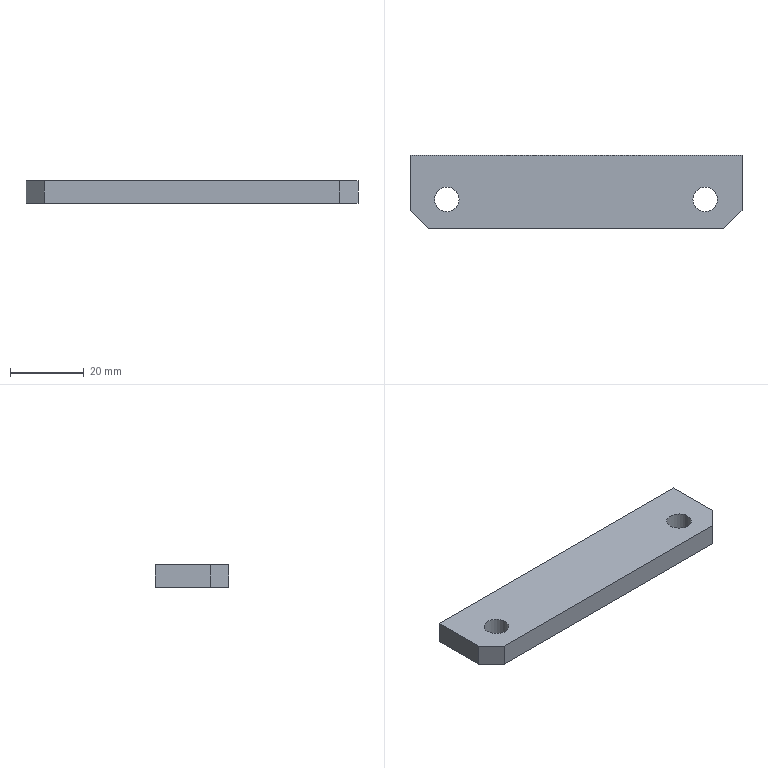Part | STEP file | weldment back plate | 1 solid | 10 faces | box 90 x 20 x 6 mm | volume 10234 mm3 | plane 8 | spline 2
STEP:
#1=CARTESIAN_POINT('',(0.,0.,0.));
#2=DIRECTION('',(0.,0.,1.));
#3=DIRECTION('',(1.,0.,0.));
#4=AXIS2_PLACEMENT_3D('',#1,#2,#3);
#5=CARTESIAN_POINT('',(90.,-15.,6.));
#6=VERTEX_POINT('',#5);
#7=CARTESIAN_POINT('',(85.,-20.,6.));
#8=VERTEX_POINT('',#7);
#9=CARTESIAN_POINT('',(90.,-15.,6.));
#10=DIRECTION('',(-0.7071,-0.7071,0.));
#11=VECTOR('',#10,1.);
#12=LINE('',#9,#11);
#13=CARTESIAN_POINT('',(87.5,-17.5,0.));
#14=DIRECTION('',(0.7071,-0.7071,0.));
#15=DIRECTION('',(0.,0.,-1.));
#16=AXIS2_PLACEMENT_3D('',#13,#14,#15);
#17=PLANE('',#16);
#18=CARTESIAN_POINT('',(-6.,3.536));
#19=DIRECTION('',(0.,-1.));
#20=VECTOR('',#19,1.);
#21=LINE('',#18,#20);
#22=(GEOMETRIC_REPRESENTATION_CONTEXT(2)PARAMETRIC_REPRESENTATION_CONTEXT()REPRESENTATION_CONTEXT('',''));
#23=DEFINITIONAL_REPRESENTATION('',(#21),#22);
#24=PCURVE('',#17,#23);
#25=CARTESIAN_POINT('',(45.,-10.,6.));
#26=DIRECTION('',(0.,0.,1.));
#27=DIRECTION('',(1.,0.,0.));
#28=AXIS2_PLACEMENT_3D('',#25,#26,#27);
#29=PLANE('',#28);
#30=CARTESIAN_POINT('',(45.,-5.));
#31=DIRECTION('',(-0.7071,-0.7071));
#32=VECTOR('',#31,1.);
#33=LINE('',#30,#32);
#34=(GEOMETRIC_REPRESENTATION_CONTEXT(2)PARAMETRIC_REPRESENTATION_CONTEXT()REPRESENTATION_CONTEXT('',''));
#35=DEFINITIONAL_REPRESENTATION('',(#33),#34);
#36=PCURVE('',#29,#35);
#37=SURFACE_CURVE('',#12,(#24,#36),.PCURVE_S1.);
#38=EDGE_CURVE('',#6,#8,#37,.T.);
#39=ORIENTED_EDGE('',*,*,#38,.T.);
#40=CARTESIAN_POINT('',(85.,-20.,0.));
#41=VERTEX_POINT('',#40);
#42=CARTESIAN_POINT('',(85.,-20.,6.));
#43=DIRECTION('',(0.,0.,-1.));
#44=VECTOR('',#43,1.);
#45=LINE('',#42,#44);
#46=CARTESIAN_POINT('',(-6.,-3.536));
#47=DIRECTION('',(1.,0.));
#48=VECTOR('',#47,1.);
#49=LINE('',#46,#48);
#50=(GEOMETRIC_REPRESENTATION_CONTEXT(2)PARAMETRIC_REPRESENTATION_CONTEXT()REPRESENTATION_CONTEXT('',''));
#51=DEFINITIONAL_REPRESENTATION('',(#49),#50);
#52=PCURVE('',#17,#51);
#53=CARTESIAN_POINT('',(90.,-20.,0.));
#54=DIRECTION('',(0.,-1.,0.));
#55=DIRECTION('',(0.,0.,-1.));
#56=AXIS2_PLACEMENT_3D('',#53,#54,#55);
#57=PLANE('',#56);
#58=CARTESIAN_POINT('',(-6.,-5.));
#59=DIRECTION('',(1.,0.));
#60=VECTOR('',#59,1.);
#61=LINE('',#58,#60);
#62=(GEOMETRIC_REPRESENTATION_CONTEXT(2)PARAMETRIC_REPRESENTATION_CONTEXT()REPRESENTATION_CONTEXT('',''));
#63=DEFINITIONAL_REPRESENTATION('',(#61),#62);
#64=PCURVE('',#57,#63);
#65=SURFACE_CURVE('',#45,(#52,#64),.PCURVE_S1.);
#66=EDGE_CURVE('',#8,#41,#65,.T.);
#67=ORIENTED_EDGE('',*,*,#66,.T.);
#68=CARTESIAN_POINT('',(90.,-15.,0.));
#69=VERTEX_POINT('',#68);
#70=CARTESIAN_POINT('',(85.,-20.,0.));
#71=DIRECTION('',(0.7071,0.7071,0.));
#72=VECTOR('',#71,1.);
#73=LINE('',#70,#72);
#74=CARTESIAN_POINT('',(0.,-3.536));
#75=DIRECTION('',(0.,1.));
#76=VECTOR('',#75,1.);
#77=LINE('',#74,#76);
#78=(GEOMETRIC_REPRESENTATION_CONTEXT(2)PARAMETRIC_REPRESENTATION_CONTEXT()REPRESENTATION_CONTEXT('',''));
#79=DEFINITIONAL_REPRESENTATION('',(#77),#78);
#80=PCURVE('',#17,#79);
#81=CARTESIAN_POINT('',(45.,-10.,0.));
#82=DIRECTION('',(0.,0.,1.));
#83=DIRECTION('',(1.,0.,0.));
#84=AXIS2_PLACEMENT_3D('',#81,#82,#83);
#85=PLANE('',#84);
#86=CARTESIAN_POINT('',(40.,-10.));
#87=DIRECTION('',(0.7071,0.7071));
#88=VECTOR('',#87,1.);
#89=LINE('',#86,#88);
#90=(GEOMETRIC_REPRESENTATION_CONTEXT(2)PARAMETRIC_REPRESENTATION_CONTEXT()REPRESENTATION_CONTEXT('',''));
#91=DEFINITIONAL_REPRESENTATION('',(#89),#90);
#92=PCURVE('',#85,#91);
#93=SURFACE_CURVE('',#73,(#80,#92),.PCURVE_S1.);
#94=EDGE_CURVE('',#41,#69,#93,.T.);
#95=ORIENTED_EDGE('',*,*,#94,.T.);
#96=CARTESIAN_POINT('',(90.,-15.,0.));
#97=DIRECTION('',(0.,0.,1.));
#98=VECTOR('',#97,1.);
#99=LINE('',#96,#98);
#100=CARTESIAN_POINT('',(0.,3.536));
#101=DIRECTION('',(-1.,0.));
#102=VECTOR('',#101,1.);
#103=LINE('',#100,#102);
#104=(GEOMETRIC_REPRESENTATION_CONTEXT(2)PARAMETRIC_REPRESENTATION_CONTEXT()REPRESENTATION_CONTEXT('',''));
#105=DEFINITIONAL_REPRESENTATION('',(#103),#104);
#106=PCURVE('',#17,#105);
#107=CARTESIAN_POINT('',(90.,0.,0.));
#108=DIRECTION('',(1.,0.,0.));
#109=DIRECTION('',(0.,0.,-1.));
#110=AXIS2_PLACEMENT_3D('',#107,#108,#109);
#111=PLANE('',#110);
#112=CARTESIAN_POINT('',(0.,-15.));
#113=DIRECTION('',(-1.,0.));
#114=VECTOR('',#113,1.);
#115=LINE('',#112,#114);
#116=(GEOMETRIC_REPRESENTATION_CONTEXT(2)PARAMETRIC_REPRESENTATION_CONTEXT()REPRESENTATION_CONTEXT('',''));
#117=DEFINITIONAL_REPRESENTATION('',(#115),#116);
#118=PCURVE('',#111,#117);
#119=SURFACE_CURVE('',#99,(#106,#118),.PCURVE_S1.);
#120=EDGE_CURVE('',#69,#6,#119,.T.);
#121=ORIENTED_EDGE('',*,*,#120,.T.);
#122=EDGE_LOOP('',(#39,#67,#95,#121));
#123=FACE_BOUND('',#122,.T.);
#124=ADVANCED_FACE('',(#123),#17,.T.);
#125=ORIENTED_EDGE('',*,*,#120,.F.);
#126=CARTESIAN_POINT('',(90.,0.,0.));
#127=VERTEX_POINT('',#126);
#128=CARTESIAN_POINT('',(90.,0.,0.));
#129=DIRECTION('',(0.,-1.,0.));
#130=VECTOR('',#129,1.);
#131=LINE('',#128,#130);
#132=CARTESIAN_POINT('',(0.,0.));
#133=DIRECTION('',(0.,-1.));
#134=VECTOR('',#133,1.);
#135=LINE('',#132,#134);
#136=(GEOMETRIC_REPRESENTATION_CONTEXT(2)PARAMETRIC_REPRESENTATION_CONTEXT()REPRESENTATION_CONTEXT('',''));
#137=DEFINITIONAL_REPRESENTATION('',(#135),#136);
#138=PCURVE('',#111,#137);
#139=CARTESIAN_POINT('',(45.,10.));
#140=DIRECTION('',(0.,-1.));
#141=VECTOR('',#140,1.);
#142=LINE('',#139,#141);
#143=(GEOMETRIC_REPRESENTATION_CONTEXT(2)PARAMETRIC_REPRESENTATION_CONTEXT()REPRESENTATION_CONTEXT('',''));
#144=DEFINITIONAL_REPRESENTATION('',(#142),#143);
#145=PCURVE('',#85,#144);
#146=SURFACE_CURVE('',#131,(#138,#145),.PCURVE_S1.);
#147=EDGE_CURVE('',#127,#69,#146,.T.);
#148=ORIENTED_EDGE('',*,*,#147,.F.);
#149=CARTESIAN_POINT('',(90.,0.,6.));
#150=VERTEX_POINT('',#149);
#151=CARTESIAN_POINT('',(90.,0.,0.));
#152=DIRECTION('',(0.,0.,1.));
#153=VECTOR('',#152,1.);
#154=LINE('',#151,#153);
#155=CARTESIAN_POINT('',(0.,0.));
#156=DIRECTION('',(-1.,0.));
#157=VECTOR('',#156,1.);
#158=LINE('',#155,#157);
#159=(GEOMETRIC_REPRESENTATION_CONTEXT(2)PARAMETRIC_REPRESENTATION_CONTEXT()REPRESENTATION_CONTEXT('',''));
#160=DEFINITIONAL_REPRESENTATION('',(#158),#159);
#161=PCURVE('',#111,#160);
#162=CARTESIAN_POINT('',(0.,0.,0.));
#163=DIRECTION('',(0.,1.,0.));
#164=DIRECTION('',(0.,0.,1.));
#165=AXIS2_PLACEMENT_3D('',#162,#163,#164);
#166=PLANE('',#165);
#167=CARTESIAN_POINT('',(0.,90.));
#168=DIRECTION('',(1.,0.));
#169=VECTOR('',#168,1.);
#170=LINE('',#167,#169);
#171=(GEOMETRIC_REPRESENTATION_CONTEXT(2)PARAMETRIC_REPRESENTATION_CONTEXT()REPRESENTATION_CONTEXT('',''));
#172=DEFINITIONAL_REPRESENTATION('',(#170),#171);
#173=PCURVE('',#166,#172);
#174=SURFACE_CURVE('',#154,(#161,#173),.PCURVE_S1.);
#175=EDGE_CURVE('',#127,#150,#174,.T.);
#176=ORIENTED_EDGE('',*,*,#175,.T.);
#177=CARTESIAN_POINT('',(90.,0.,6.));
#178=DIRECTION('',(0.,-1.,0.));
#179=VECTOR('',#178,1.);
#180=LINE('',#177,#179);
#181=CARTESIAN_POINT('',(-6.,0.));
#182=DIRECTION('',(0.,-1.));
#183=VECTOR('',#182,1.);
#184=LINE('',#181,#183);
#185=(GEOMETRIC_REPRESENTATION_CONTEXT(2)PARAMETRIC_REPRESENTATION_CONTEXT()REPRESENTATION_CONTEXT('',''));
#186=DEFINITIONAL_REPRESENTATION('',(#184),#185);
#187=PCURVE('',#111,#186);
#188=CARTESIAN_POINT('',(45.,10.));
#189=DIRECTION('',(0.,-1.));
#190=VECTOR('',#189,1.);
#191=LINE('',#188,#190);
#192=(GEOMETRIC_REPRESENTATION_CONTEXT(2)PARAMETRIC_REPRESENTATION_CONTEXT()REPRESENTATION_CONTEXT('',''));
#193=DEFINITIONAL_REPRESENTATION('',(#191),#192);
#194=PCURVE('',#29,#193);
#195=SURFACE_CURVE('',#180,(#187,#194),.PCURVE_S1.);
#196=EDGE_CURVE('',#150,#6,#195,.T.);
#197=ORIENTED_EDGE('',*,*,#196,.T.);
#198=EDGE_LOOP('',(#125,#148,#176,#197));
#199=FACE_BOUND('',#198,.T.);
#200=ADVANCED_FACE('',(#199),#111,.T.);
#201=ORIENTED_EDGE('',*,*,#94,.F.);
#202=CARTESIAN_POINT('',(5.,-20.,0.));
#203=VERTEX_POINT('',#202);
#204=CARTESIAN_POINT('',(85.,-20.,0.));
#205=DIRECTION('',(-1.,0.,0.));
#206=VECTOR('',#205,1.);
#207=LINE('',#204,#206);
#208=CARTESIAN_POINT('',(40.,-10.));
#209=DIRECTION('',(-1.,0.));
#210=VECTOR('',#209,1.);
#211=LINE('',#208,#210);
#212=(GEOMETRIC_REPRESENTATION_CONTEXT(2)PARAMETRIC_REPRESENTATION_CONTEXT()REPRESENTATION_CONTEXT('',''));
#213=DEFINITIONAL_REPRESENTATION('',(#211),#212);
#214=PCURVE('',#85,#213);
#215=CARTESIAN_POINT('',(0.,-5.));
#216=DIRECTION('',(0.,-1.));
#217=VECTOR('',#216,1.);
#218=LINE('',#215,#217);
#219=(GEOMETRIC_REPRESENTATION_CONTEXT(2)PARAMETRIC_REPRESENTATION_CONTEXT()REPRESENTATION_CONTEXT('',''));
#220=DEFINITIONAL_REPRESENTATION('',(#218),#219);
#221=PCURVE('',#57,#220);
#222=SURFACE_CURVE('',#207,(#214,#221),.PCURVE_S1.);
#223=EDGE_CURVE('',#41,#203,#222,.T.);
#224=ORIENTED_EDGE('',*,*,#223,.T.);
#225=CARTESIAN_POINT('',(0.,-15.,0.));
#226=VERTEX_POINT('',#225);
#227=CARTESIAN_POINT('',(0.,-15.,0.));
#228=DIRECTION('',(0.7071,-0.7071,0.));
#229=VECTOR('',#228,1.);
#230=LINE('',#227,#229);
#231=CARTESIAN_POINT('',(-45.,-5.));
#232=DIRECTION('',(0.7071,-0.7071));
#233=VECTOR('',#232,1.);
#234=LINE('',#231,#233);
#235=(GEOMETRIC_REPRESENTATION_CONTEXT(2)PARAMETRIC_REPRESENTATION_CONTEXT()REPRESENTATION_CONTEXT('',''));
#236=DEFINITIONAL_REPRESENTATION('',(#234),#235);
#237=PCURVE('',#85,#236);
#238=CARTESIAN_POINT('',(2.5,-17.5,0.));
#239=DIRECTION('',(-0.7071,-0.7071,0.));
#240=DIRECTION('',(0.,0.,1.));
#241=AXIS2_PLACEMENT_3D('',#238,#239,#240);
#242=PLANE('',#241);
#243=CARTESIAN_POINT('',(0.,3.536));
#244=DIRECTION('',(0.,-1.));
#245=VECTOR('',#244,1.);
#246=LINE('',#243,#245);
#247=(GEOMETRIC_REPRESENTATION_CONTEXT(2)PARAMETRIC_REPRESENTATION_CONTEXT()REPRESENTATION_CONTEXT('',''));
#248=DEFINITIONAL_REPRESENTATION('',(#246),#247);
#249=PCURVE('',#242,#248);
#250=SURFACE_CURVE('',#230,(#237,#249),.PCURVE_S1.);
#251=EDGE_CURVE('',#226,#203,#250,.T.);
#252=ORIENTED_EDGE('',*,*,#251,.F.);
#253=CARTESIAN_POINT('',(0.,0.,0.));
#254=VERTEX_POINT('',#253);
#255=CARTESIAN_POINT('',(0.,-15.,0.));
#256=DIRECTION('',(0.,1.,0.));
#257=VECTOR('',#256,1.);
#258=LINE('',#255,#257);
#259=CARTESIAN_POINT('',(-45.,-5.));
#260=DIRECTION('',(0.,1.));
#261=VECTOR('',#260,1.);
#262=LINE('',#259,#261);
#263=(GEOMETRIC_REPRESENTATION_CONTEXT(2)PARAMETRIC_REPRESENTATION_CONTEXT()REPRESENTATION_CONTEXT('',''));
#264=DEFINITIONAL_REPRESENTATION('',(#262),#263);
#265=PCURVE('',#85,#264);
#266=CARTESIAN_POINT('',(0.,-20.,0.));
#267=DIRECTION('',(-1.,0.,0.));
#268=DIRECTION('',(0.,0.,1.));
#269=AXIS2_PLACEMENT_3D('',#266,#267,#268);
#270=PLANE('',#269);
#271=CARTESIAN_POINT('',(0.,5.));
#272=DIRECTION('',(0.,1.));
#273=VECTOR('',#272,1.);
#274=LINE('',#271,#273);
#275=(GEOMETRIC_REPRESENTATION_CONTEXT(2)PARAMETRIC_REPRESENTATION_CONTEXT()REPRESENTATION_CONTEXT('',''));
#276=DEFINITIONAL_REPRESENTATION('',(#274),#275);
#277=PCURVE('',#270,#276);
#278=SURFACE_CURVE('',#258,(#265,#277),.PCURVE_S1.);
#279=EDGE_CURVE('',#226,#254,#278,.T.);
#280=ORIENTED_EDGE('',*,*,#279,.T.);
#281=CARTESIAN_POINT('',(0.,0.,0.));
#282=DIRECTION('',(1.,0.,0.));
#283=VECTOR('',#282,1.);
#284=LINE('',#281,#283);
#285=CARTESIAN_POINT('',(-45.,10.));
#286=DIRECTION('',(1.,0.));
#287=VECTOR('',#286,1.);
#288=LINE('',#285,#287);
#289=(GEOMETRIC_REPRESENTATION_CONTEXT(2)PARAMETRIC_REPRESENTATION_CONTEXT()REPRESENTATION_CONTEXT('',''));
#290=DEFINITIONAL_REPRESENTATION('',(#288),#289);
#291=PCURVE('',#85,#290);
#292=CARTESIAN_POINT('',(0.,0.));
#293=DIRECTION('',(0.,1.));
#294=VECTOR('',#293,1.);
#295=LINE('',#292,#294);
#296=(GEOMETRIC_REPRESENTATION_CONTEXT(2)PARAMETRIC_REPRESENTATION_CONTEXT()REPRESENTATION_CONTEXT('',''));
#297=DEFINITIONAL_REPRESENTATION('',(#295),#296);
#298=PCURVE('',#166,#297);
#299=SURFACE_CURVE('',#284,(#291,#298),.PCURVE_S1.);
#300=EDGE_CURVE('',#254,#127,#299,.T.);
#301=ORIENTED_EDGE('',*,*,#300,.T.);
#302=ORIENTED_EDGE('',*,*,#147,.T.);
#303=EDGE_LOOP('',(#201,#224,#252,#280,#301,#302));
#304=FACE_BOUND('',#303,.T.);
#305=CARTESIAN_POINT('',(76.677,-12.,0.));
#306=VERTEX_POINT('',#305);
#307=CARTESIAN_POINT('',(80.,-12.,0.));
#308=DIRECTION('',(0.,0.,1.));
#309=DIRECTION('',(1.,0.,0.));
#310=AXIS2_PLACEMENT_3D('',#307,#308,#309);
#311=CIRCLE('',#310,3.324);
#312=CARTESIAN_POINT('',(35.,-2.));
#313=DIRECTION('',(1.,0.));
#314=AXIS2_PLACEMENT_2D('',#312,#313);
#315=CIRCLE('',#314,3.324);
#316=(GEOMETRIC_REPRESENTATION_CONTEXT(2)PARAMETRIC_REPRESENTATION_CONTEXT()REPRESENTATION_CONTEXT('',''));
#317=DEFINITIONAL_REPRESENTATION('',(#315),#316);
#318=PCURVE('',#85,#317);
#319=CARTESIAN_POINT('',(76.677,-12.,6.));
#320=CARTESIAN_POINT('',(76.677,-15.323,6.));
#321=CARTESIAN_POINT('',(80.,-15.323,6.));
#322=CARTESIAN_POINT('',(83.323,-15.323,6.));
#323=CARTESIAN_POINT('',(83.323,-12.,6.));
#324=CARTESIAN_POINT('',(83.323,-8.677,6.));
#325=CARTESIAN_POINT('',(80.,-8.677,6.));
#326=CARTESIAN_POINT('',(76.677,-8.677,6.));
#327=CARTESIAN_POINT('',(76.677,-12.,6.));
#328=CARTESIAN_POINT('',(76.677,-12.,0.));
#329=CARTESIAN_POINT('',(76.677,-15.323,0.));
#330=CARTESIAN_POINT('',(80.,-15.323,0.));
#331=CARTESIAN_POINT('',(83.323,-15.323,0.));
#332=CARTESIAN_POINT('',(83.323,-12.,0.));
#333=CARTESIAN_POINT('',(83.323,-8.677,0.));
#334=CARTESIAN_POINT('',(80.,-8.677,0.));
#335=CARTESIAN_POINT('',(76.677,-8.677,0.));
#336=CARTESIAN_POINT('',(76.677,-12.,0.));
#337=(BOUNDED_SURFACE()B_SPLINE_SURFACE(1,2,((#319,#320,#321,#322,#323,#324,#325,#326,#327),(#328,#329,#330,#331,#332,#333,#334,#335,#336)),.UNSPECIFIED.,.F.,.T.,.F.)B_SPLINE_SURFACE_WITH_KNOTS((2,2),(1,2,2,2,2,2,1),(-27.799,-25.994),(-5.221,0.,5.221,10.441,15.662,20.882,26.103),.UNSPECIFIED.)GEOMETRIC_REPRESENTATION_ITEM()RATIONAL_B_SPLINE_SURFACE(((1.,0.7071,1.,0.7071,1.,0.7071,1.,0.7071,1.),(1.,0.7071,1.,0.7071,1.,0.7071,1.,0.7071,1.)))REPRESENTATION_ITEM('')SURFACE());
#338=CARTESIAN_POINT('',(-25.994,0.));
#339=CARTESIAN_POINT('',(-25.994,0.3505));
#340=CARTESIAN_POINT('',(-25.994,1.014));
#341=CARTESIAN_POINT('',(-25.994,1.937));
#342=CARTESIAN_POINT('',(-25.994,2.834));
#343=CARTESIAN_POINT('',(-25.994,3.74));
#344=CARTESIAN_POINT('',(-25.994,4.688));
#345=CARTESIAN_POINT('',(-25.994,5.753));
#346=CARTESIAN_POINT('',(-25.994,6.701));
#347=CARTESIAN_POINT('',(-25.994,7.607));
#348=CARTESIAN_POINT('',(-25.994,8.505));
#349=CARTESIAN_POINT('',(-25.994,9.422));
#350=CARTESIAN_POINT('',(-25.994,10.441));
#351=CARTESIAN_POINT('',(-25.994,11.46));
#352=CARTESIAN_POINT('',(-25.994,12.377));
#353=CARTESIAN_POINT('',(-25.994,13.275));
#354=CARTESIAN_POINT('',(-25.994,14.181));
#355=CARTESIAN_POINT('',(-25.994,15.129));
#356=CARTESIAN_POINT('',(-25.994,16.194));
#357=CARTESIAN_POINT('',(-25.994,17.142));
#358=CARTESIAN_POINT('',(-25.994,18.049));
#359=CARTESIAN_POINT('',(-25.994,18.945));
#360=CARTESIAN_POINT('',(-25.994,19.868));
#361=CARTESIAN_POINT('',(-25.994,20.532));
#362=CARTESIAN_POINT('',(-25.994,20.882));
#363=B_SPLINE_CURVE_WITH_KNOTS('',3,(#338,#339,#340,#341,#342,#343,#344,#345,#346,#347,#348,#349,#350,#351,#352,#353,#354,#355,#356,#357,#358,#359,#360,#361,#362),.UNSPECIFIED.,.F.,.F.,(4,1,1,1,1,1,1,1,1,1,1,1,1,1,1,1,1,1,1,1,1,1,4),(3.142,3.427,3.713,3.998,4.284,4.57,4.855,5.141,5.426,5.712,5.998,6.283,6.569,6.854,7.14,7.426,7.711,7.997,8.282,8.568,8.854,9.139,9.425),.QUASI_UNIFORM_KNOTS.);
#364=(GEOMETRIC_REPRESENTATION_CONTEXT(2)PARAMETRIC_REPRESENTATION_CONTEXT()REPRESENTATION_CONTEXT('',''));
#365=DEFINITIONAL_REPRESENTATION('',(#363),#364);
#366=PCURVE('',#337,#365);
#367=SURFACE_CURVE('',#311,(#318,#366),.PCURVE_S1.);
#368=EDGE_CURVE('',#306,#306,#367,.T.);
#369=ORIENTED_EDGE('',*,*,#368,.T.);
#370=EDGE_LOOP('',(#369));
#371=FACE_BOUND('',#370,.T.);
#372=CARTESIAN_POINT('',(6.676,-12.,0.));
#373=VERTEX_POINT('',#372);
#374=CARTESIAN_POINT('',(10.,-12.,0.));
#375=DIRECTION('',(0.,0.,1.));
#376=DIRECTION('',(1.,0.,0.));
#377=AXIS2_PLACEMENT_3D('',#374,#375,#376);
#378=CIRCLE('',#377,3.324);
#379=CARTESIAN_POINT('',(-35.,-2.));
#380=DIRECTION('',(1.,0.));
#381=AXIS2_PLACEMENT_2D('',#379,#380);
#382=CIRCLE('',#381,3.324);
#383=(GEOMETRIC_REPRESENTATION_CONTEXT(2)PARAMETRIC_REPRESENTATION_CONTEXT()REPRESENTATION_CONTEXT('',''));
#384=DEFINITIONAL_REPRESENTATION('',(#382),#383);
#385=PCURVE('',#85,#384);
#386=CARTESIAN_POINT('',(6.676,-12.,6.));
#387=CARTESIAN_POINT('',(6.676,-15.323,6.));
#388=CARTESIAN_POINT('',(10.,-15.323,6.));
#389=CARTESIAN_POINT('',(13.323,-15.323,6.));
#390=CARTESIAN_POINT('',(13.323,-12.,6.));
#391=CARTESIAN_POINT('',(13.323,-8.677,6.));
#392=CARTESIAN_POINT('',(10.,-8.677,6.));
#393=CARTESIAN_POINT('',(6.676,-8.677,6.));
#394=CARTESIAN_POINT('',(6.676,-12.,6.));
#395=CARTESIAN_POINT('',(6.676,-12.,0.));
#396=CARTESIAN_POINT('',(6.676,-15.323,0.));
#397=CARTESIAN_POINT('',(10.,-15.323,0.));
#398=CARTESIAN_POINT('',(13.323,-15.323,0.));
#399=CARTESIAN_POINT('',(13.323,-12.,0.));
#400=CARTESIAN_POINT('',(13.323,-8.677,0.));
#401=CARTESIAN_POINT('',(10.,-8.677,0.));
#402=CARTESIAN_POINT('',(6.676,-8.677,0.));
#403=CARTESIAN_POINT('',(6.676,-12.,0.));
#404=(BOUNDED_SURFACE()B_SPLINE_SURFACE(1,2,((#386,#387,#388,#389,#390,#391,#392,#393,#394),(#395,#396,#397,#398,#399,#400,#401,#402,#403)),.UNSPECIFIED.,.F.,.T.,.F.)B_SPLINE_SURFACE_WITH_KNOTS((2,2),(1,2,2,2,2,2,1),(-27.799,-25.994),(-5.221,0.,5.221,10.441,15.662,20.882,26.103),.UNSPECIFIED.)GEOMETRIC_REPRESENTATION_ITEM()RATIONAL_B_SPLINE_SURFACE(((1.,0.7071,1.,0.7071,1.,0.7071,1.,0.7071,1.),(1.,0.7071,1.,0.7071,1.,0.7071,1.,0.7071,1.)))REPRESENTATION_ITEM('')SURFACE());
#405=CARTESIAN_POINT('',(-25.994,0.));
#406=CARTESIAN_POINT('',(-25.994,0.3505));
#407=CARTESIAN_POINT('',(-25.994,1.014));
#408=CARTESIAN_POINT('',(-25.994,1.937));
#409=CARTESIAN_POINT('',(-25.994,2.834));
#410=CARTESIAN_POINT('',(-25.994,3.74));
#411=CARTESIAN_POINT('',(-25.994,4.688));
#412=CARTESIAN_POINT('',(-25.994,5.753));
#413=CARTESIAN_POINT('',(-25.994,6.701));
#414=CARTESIAN_POINT('',(-25.994,7.607));
#415=CARTESIAN_POINT('',(-25.994,8.505));
#416=CARTESIAN_POINT('',(-25.994,9.422));
#417=CARTESIAN_POINT('',(-25.994,10.441));
#418=CARTESIAN_POINT('',(-25.994,11.46));
#419=CARTESIAN_POINT('',(-25.994,12.377));
#420=CARTESIAN_POINT('',(-25.994,13.275));
#421=CARTESIAN_POINT('',(-25.994,14.181));
#422=CARTESIAN_POINT('',(-25.994,15.129));
#423=CARTESIAN_POINT('',(-25.994,16.194));
#424=CARTESIAN_POINT('',(-25.994,17.142));
#425=CARTESIAN_POINT('',(-25.994,18.049));
#426=CARTESIAN_POINT('',(-25.994,18.945));
#427=CARTESIAN_POINT('',(-25.994,19.868));
#428=CARTESIAN_POINT('',(-25.994,20.532));
#429=CARTESIAN_POINT('',(-25.994,20.882));
#430=B_SPLINE_CURVE_WITH_KNOTS('',3,(#405,#406,#407,#408,#409,#410,#411,#412,#413,#414,#415,#416,#417,#418,#419,#420,#421,#422,#423,#424,#425,#426,#427,#428,#429),.UNSPECIFIED.,.F.,.F.,(4,1,1,1,1,1,1,1,1,1,1,1,1,1,1,1,1,1,1,1,1,1,4),(3.142,3.427,3.713,3.998,4.284,4.57,4.855,5.141,5.426,5.712,5.998,6.283,6.569,6.854,7.14,7.426,7.711,7.997,8.282,8.568,8.854,9.139,9.425),.QUASI_UNIFORM_KNOTS.);
#431=(GEOMETRIC_REPRESENTATION_CONTEXT(2)PARAMETRIC_REPRESENTATION_CONTEXT()REPRESENTATION_CONTEXT('',''));
#432=DEFINITIONAL_REPRESENTATION('',(#430),#431);
#433=PCURVE('',#404,#432);
#434=SURFACE_CURVE('',#378,(#385,#433),.PCURVE_S1.);
#435=EDGE_CURVE('',#373,#373,#434,.T.);
#436=ORIENTED_EDGE('',*,*,#435,.T.);
#437=EDGE_LOOP('',(#436));
#438=FACE_BOUND('',#437,.T.);
#439=ADVANCED_FACE('',(#304,#371,#438),#85,.F.);
#440=CARTESIAN_POINT('',(5.,-20.,6.));
#441=VERTEX_POINT('',#440);
#442=CARTESIAN_POINT('',(0.,-15.,6.));
#443=VERTEX_POINT('',#442);
#444=CARTESIAN_POINT('',(5.,-20.,6.));
#445=DIRECTION('',(-0.7071,0.7071,0.));
#446=VECTOR('',#445,1.);
#447=LINE('',#444,#446);
#448=CARTESIAN_POINT('',(6.,-3.536));
#449=DIRECTION('',(0.,1.));
#450=VECTOR('',#449,1.);
#451=LINE('',#448,#450);
#452=(GEOMETRIC_REPRESENTATION_CONTEXT(2)PARAMETRIC_REPRESENTATION_CONTEXT()REPRESENTATION_CONTEXT('',''));
#453=DEFINITIONAL_REPRESENTATION('',(#451),#452);
#454=PCURVE('',#242,#453);
#455=CARTESIAN_POINT('',(-40.,-10.));
#456=DIRECTION('',(-0.7071,0.7071));
#457=VECTOR('',#456,1.);
#458=LINE('',#455,#457);
#459=(GEOMETRIC_REPRESENTATION_CONTEXT(2)PARAMETRIC_REPRESENTATION_CONTEXT()REPRESENTATION_CONTEXT('',''));
#460=DEFINITIONAL_REPRESENTATION('',(#458),#459);
#461=PCURVE('',#29,#460);
#462=SURFACE_CURVE('',#447,(#454,#461),.PCURVE_S1.);
#463=EDGE_CURVE('',#441,#443,#462,.T.);
#464=ORIENTED_EDGE('',*,*,#463,.T.);
#465=CARTESIAN_POINT('',(0.,-15.,6.));
#466=DIRECTION('',(0.,0.,-1.));
#467=VECTOR('',#466,1.);
#468=LINE('',#465,#467);
#469=CARTESIAN_POINT('',(6.,3.536));
#470=DIRECTION('',(-1.,0.));
#471=VECTOR('',#470,1.);
#472=LINE('',#469,#471);
#473=(GEOMETRIC_REPRESENTATION_CONTEXT(2)PARAMETRIC_REPRESENTATION_CONTEXT()REPRESENTATION_CONTEXT('',''));
#474=DEFINITIONAL_REPRESENTATION('',(#472),#473);
#475=PCURVE('',#242,#474);
#476=CARTESIAN_POINT('',(6.,5.));
#477=DIRECTION('',(-1.,0.));
#478=VECTOR('',#477,1.);
#479=LINE('',#476,#478);
#480=(GEOMETRIC_REPRESENTATION_CONTEXT(2)PARAMETRIC_REPRESENTATION_CONTEXT()REPRESENTATION_CONTEXT('',''));
#481=DEFINITIONAL_REPRESENTATION('',(#479),#480);
#482=PCURVE('',#270,#481);
#483=SURFACE_CURVE('',#468,(#475,#482),.PCURVE_S1.);
#484=EDGE_CURVE('',#443,#226,#483,.T.);
#485=ORIENTED_EDGE('',*,*,#484,.T.);
#486=ORIENTED_EDGE('',*,*,#251,.T.);
#487=CARTESIAN_POINT('',(5.,-20.,0.));
#488=DIRECTION('',(0.,0.,1.));
#489=VECTOR('',#488,1.);
#490=LINE('',#487,#489);
#491=CARTESIAN_POINT('',(0.,-3.536));
#492=DIRECTION('',(1.,0.));
#493=VECTOR('',#492,1.);
#494=LINE('',#491,#493);
#495=(GEOMETRIC_REPRESENTATION_CONTEXT(2)PARAMETRIC_REPRESENTATION_CONTEXT()REPRESENTATION_CONTEXT('',''));
#496=DEFINITIONAL_REPRESENTATION('',(#494),#495);
#497=PCURVE('',#242,#496);
#498=CARTESIAN_POINT('',(0.,-85.));
#499=DIRECTION('',(-1.,0.));
#500=VECTOR('',#499,1.);
#501=LINE('',#498,#500);
#502=(GEOMETRIC_REPRESENTATION_CONTEXT(2)PARAMETRIC_REPRESENTATION_CONTEXT()REPRESENTATION_CONTEXT('',''));
#503=DEFINITIONAL_REPRESENTATION('',(#501),#502);
#504=PCURVE('',#57,#503);
#505=SURFACE_CURVE('',#490,(#497,#504),.PCURVE_S1.);
#506=EDGE_CURVE('',#203,#441,#505,.T.);
#507=ORIENTED_EDGE('',*,*,#506,.T.);
#508=EDGE_LOOP('',(#464,#485,#486,#507));
#509=FACE_BOUND('',#508,.T.);
#510=ADVANCED_FACE('',(#509),#242,.T.);
#511=ORIENTED_EDGE('',*,*,#484,.F.);
#512=CARTESIAN_POINT('',(0.,0.,6.));
#513=VERTEX_POINT('',#512);
#514=CARTESIAN_POINT('',(0.,-15.,6.));
#515=DIRECTION('',(0.,1.,0.));
#516=VECTOR('',#515,1.);
#517=LINE('',#514,#516);
#518=CARTESIAN_POINT('',(6.,5.));
#519=DIRECTION('',(0.,1.));
#520=VECTOR('',#519,1.);
#521=LINE('',#518,#520);
#522=(GEOMETRIC_REPRESENTATION_CONTEXT(2)PARAMETRIC_REPRESENTATION_CONTEXT()REPRESENTATION_CONTEXT('',''));
#523=DEFINITIONAL_REPRESENTATION('',(#521),#522);
#524=PCURVE('',#270,#523);
#525=CARTESIAN_POINT('',(-45.,-5.));
#526=DIRECTION('',(0.,1.));
#527=VECTOR('',#526,1.);
#528=LINE('',#525,#527);
#529=(GEOMETRIC_REPRESENTATION_CONTEXT(2)PARAMETRIC_REPRESENTATION_CONTEXT()REPRESENTATION_CONTEXT('',''));
#530=DEFINITIONAL_REPRESENTATION('',(#528),#529);
#531=PCURVE('',#29,#530);
#532=SURFACE_CURVE('',#517,(#524,#531),.PCURVE_S1.);
#533=EDGE_CURVE('',#443,#513,#532,.T.);
#534=ORIENTED_EDGE('',*,*,#533,.T.);
#535=CARTESIAN_POINT('',(0.,0.,0.));
#536=DIRECTION('',(0.,0.,1.));
#537=VECTOR('',#536,1.);
#538=LINE('',#535,#537);
#539=CARTESIAN_POINT('',(0.,20.));
#540=DIRECTION('',(1.,0.));
#541=VECTOR('',#540,1.);
#542=LINE('',#539,#541);
#543=(GEOMETRIC_REPRESENTATION_CONTEXT(2)PARAMETRIC_REPRESENTATION_CONTEXT()REPRESENTATION_CONTEXT('',''));
#544=DEFINITIONAL_REPRESENTATION('',(#542),#543);
#545=PCURVE('',#270,#544);
#546=CARTESIAN_POINT('',(0.,0.));
#547=DIRECTION('',(1.,0.));
#548=VECTOR('',#547,1.);
#549=LINE('',#546,#548);
#550=(GEOMETRIC_REPRESENTATION_CONTEXT(2)PARAMETRIC_REPRESENTATION_CONTEXT()REPRESENTATION_CONTEXT('',''));
#551=DEFINITIONAL_REPRESENTATION('',(#549),#550);
#552=PCURVE('',#166,#551);
#553=SURFACE_CURVE('',#538,(#545,#552),.PCURVE_S1.);
#554=EDGE_CURVE('',#254,#513,#553,.T.);
#555=ORIENTED_EDGE('',*,*,#554,.F.);
#556=ORIENTED_EDGE('',*,*,#279,.F.);
#557=EDGE_LOOP('',(#511,#534,#555,#556));
#558=FACE_BOUND('',#557,.T.);
#559=ADVANCED_FACE('',(#558),#270,.T.);
#560=ORIENTED_EDGE('',*,*,#368,.T.);
#561=CARTESIAN_POINT('',(76.677,-12.,6.));
#562=VERTEX_POINT('',#561);
#563=CARTESIAN_POINT('',(76.677,-12.,6.));
#564=CARTESIAN_POINT('',(76.677,-12.,0.));
#565=B_SPLINE_CURVE_WITH_KNOTS('',1,(#563,#564),.UNSPECIFIED.,.F.,.F.,(2,2),(-27.799,-25.994),.PIECEWISE_BEZIER_KNOTS.);
#566=CARTESIAN_POINT('',(0.,20.882));
#567=DIRECTION('',(1.,0.));
#568=VECTOR('',#567,1.);
#569=LINE('',#566,#568);
#570=(GEOMETRIC_REPRESENTATION_CONTEXT(2)PARAMETRIC_REPRESENTATION_CONTEXT()REPRESENTATION_CONTEXT('',''));
#571=DEFINITIONAL_REPRESENTATION('',(#569),#570);
#572=PCURVE('',#337,#571);
#573=CARTESIAN_POINT('',(0.,0.));
#574=DIRECTION('',(1.,0.));
#575=VECTOR('',#574,1.);
#576=LINE('',#573,#575);
#577=(GEOMETRIC_REPRESENTATION_CONTEXT(2)PARAMETRIC_REPRESENTATION_CONTEXT()REPRESENTATION_CONTEXT('',''));
#578=DEFINITIONAL_REPRESENTATION('',(#576),#577);
#579=PCURVE('',#337,#578);
#580=SEAM_CURVE('',#565,(#572,#579),.PCURVE_S1.);
#581=EDGE_CURVE('',#562,#306,#580,.T.);
#582=ORIENTED_EDGE('',*,*,#581,.F.);
#583=CARTESIAN_POINT('',(83.323,-12.,6.));
#584=VERTEX_POINT('',#583);
#585=CARTESIAN_POINT('',(80.,-12.,6.));
#586=DIRECTION('',(0.,0.,-1.));
#587=DIRECTION('',(1.,0.,0.));
#588=AXIS2_PLACEMENT_3D('',#585,#586,#587);
#589=CIRCLE('',#588,3.324);
#590=CARTESIAN_POINT('',(-27.799,31.323));
#591=CARTESIAN_POINT('',(-27.799,30.973));
#592=CARTESIAN_POINT('',(-27.799,30.31));
#593=CARTESIAN_POINT('',(-27.799,29.386));
#594=CARTESIAN_POINT('',(-27.799,28.49));
#595=CARTESIAN_POINT('',(-27.799,27.583));
#596=CARTESIAN_POINT('',(-27.799,26.635));
#597=CARTESIAN_POINT('',(-27.799,25.57));
#598=CARTESIAN_POINT('',(-27.799,24.622));
#599=CARTESIAN_POINT('',(-27.799,23.716));
#600=CARTESIAN_POINT('',(-27.799,22.818));
#601=CARTESIAN_POINT('',(-27.799,21.901));
#602=CARTESIAN_POINT('',(-27.799,20.882));
#603=CARTESIAN_POINT('',(-27.799,19.863));
#604=CARTESIAN_POINT('',(-27.799,18.946));
#605=CARTESIAN_POINT('',(-27.799,18.048));
#606=CARTESIAN_POINT('',(-27.799,17.142));
#607=CARTESIAN_POINT('',(-27.799,16.194));
#608=CARTESIAN_POINT('',(-27.799,15.129));
#609=CARTESIAN_POINT('',(-27.799,14.181));
#610=CARTESIAN_POINT('',(-27.799,13.275));
#611=CARTESIAN_POINT('',(-27.799,12.378));
#612=CARTESIAN_POINT('',(-27.799,11.455));
#613=CARTESIAN_POINT('',(-27.799,10.792));
#614=CARTESIAN_POINT('',(-27.799,10.441));
#615=B_SPLINE_CURVE_WITH_KNOTS('',3,(#590,#591,#592,#593,#594,#595,#596,#597,#598,#599,#600,#601,#602,#603,#604,#605,#606,#607,#608,#609,#610,#611,#612,#613,#614),.UNSPECIFIED.,.F.,.F.,(4,1,1,1,1,1,1,1,1,1,1,1,1,1,1,1,1,1,1,1,1,1,4),(0.,0.2856,0.5712,0.8568,1.142,1.428,1.714,1.999,2.285,2.57,2.856,3.142,3.427,3.713,3.998,4.284,4.57,4.855,5.141,5.426,5.712,5.998,6.283),.QUASI_UNIFORM_KNOTS.);
#616=(GEOMETRIC_REPRESENTATION_CONTEXT(2)PARAMETRIC_REPRESENTATION_CONTEXT()REPRESENTATION_CONTEXT('',''));
#617=DEFINITIONAL_REPRESENTATION('',(#615),#616);
#618=PCURVE('',#337,#617);
#619=CARTESIAN_POINT('',(38.324,-2.));
#620=CARTESIAN_POINT('',(38.324,-7.756));
#621=CARTESIAN_POINT('',(33.338,-4.878));
#622=CARTESIAN_POINT('',(28.353,-2.));
#623=CARTESIAN_POINT('',(33.338,0.8782));
#624=CARTESIAN_POINT('',(38.324,3.756));
#625=CARTESIAN_POINT('',(38.324,-2.));
#626=(BOUNDED_CURVE()B_SPLINE_CURVE(2,(#619,#620,#621,#622,#623,#624,#625),.UNSPECIFIED.,.T.,.F.)B_SPLINE_CURVE_WITH_KNOTS((1,2,2,2,2,1),(-2.094,0.,2.094,4.189,6.283,8.378),.UNSPECIFIED.)CURVE()GEOMETRIC_REPRESENTATION_ITEM()RATIONAL_B_SPLINE_CURVE((1.,0.5,1.,0.5,1.,0.5,1.))REPRESENTATION_ITEM(''));
#627=(GEOMETRIC_REPRESENTATION_CONTEXT(2)PARAMETRIC_REPRESENTATION_CONTEXT()REPRESENTATION_CONTEXT('',''));
#628=DEFINITIONAL_REPRESENTATION('',(#626),#627);
#629=PCURVE('',#29,#628);
#630=SURFACE_CURVE('',#589,(#618,#629),.PCURVE_S1.);
#631=EDGE_CURVE('',#562,#584,#630,.T.);
#632=ORIENTED_EDGE('',*,*,#631,.T.);
#633=CARTESIAN_POINT('',(80.,-12.,6.));
#634=DIRECTION('',(0.,0.,-1.));
#635=DIRECTION('',(1.,0.,0.));
#636=AXIS2_PLACEMENT_3D('',#633,#634,#635);
#637=CIRCLE('',#636,3.324);
#638=CARTESIAN_POINT('',(-27.799,10.441));
#639=CARTESIAN_POINT('',(-27.799,10.091));
#640=CARTESIAN_POINT('',(-27.799,9.427));
#641=CARTESIAN_POINT('',(-27.799,8.504));
#642=CARTESIAN_POINT('',(-27.799,7.608));
#643=CARTESIAN_POINT('',(-27.799,6.701));
#644=CARTESIAN_POINT('',(-27.799,5.753));
#645=CARTESIAN_POINT('',(-27.799,4.688));
#646=CARTESIAN_POINT('',(-27.799,3.74));
#647=CARTESIAN_POINT('',(-27.799,2.834));
#648=CARTESIAN_POINT('',(-27.799,1.936));
#649=CARTESIAN_POINT('',(-27.799,1.019));
#650=CARTESIAN_POINT('',(-27.799,0.));
#651=CARTESIAN_POINT('',(-27.799,-1.019));
#652=CARTESIAN_POINT('',(-27.799,-1.936));
#653=CARTESIAN_POINT('',(-27.799,-2.834));
#654=CARTESIAN_POINT('',(-27.799,-3.74));
#655=CARTESIAN_POINT('',(-27.799,-4.688));
#656=CARTESIAN_POINT('',(-27.799,-5.753));
#657=CARTESIAN_POINT('',(-27.799,-6.701));
#658=CARTESIAN_POINT('',(-27.799,-7.608));
#659=CARTESIAN_POINT('',(-27.799,-8.504));
#660=CARTESIAN_POINT('',(-27.799,-9.427));
#661=CARTESIAN_POINT('',(-27.799,-10.091));
#662=CARTESIAN_POINT('',(-27.799,-10.441));
#663=B_SPLINE_CURVE_WITH_KNOTS('',3,(#638,#639,#640,#641,#642,#643,#644,#645,#646,#647,#648,#649,#650,#651,#652,#653,#654,#655,#656,#657,#658,#659,#660,#661,#662),.UNSPECIFIED.,.F.,.F.,(4,1,1,1,1,1,1,1,1,1,1,1,1,1,1,1,1,1,1,1,1,1,4),(0.,0.2856,0.5712,0.8568,1.142,1.428,1.714,1.999,2.285,2.57,2.856,3.142,3.427,3.713,3.998,4.284,4.57,4.855,5.141,5.426,5.712,5.998,6.283),.QUASI_UNIFORM_KNOTS.);
#664=(GEOMETRIC_REPRESENTATION_CONTEXT(2)PARAMETRIC_REPRESENTATION_CONTEXT()REPRESENTATION_CONTEXT('',''));
#665=DEFINITIONAL_REPRESENTATION('',(#663),#664);
#666=PCURVE('',#337,#665);
#667=CARTESIAN_POINT('',(38.324,-2.));
#668=CARTESIAN_POINT('',(38.324,-7.756));
#669=CARTESIAN_POINT('',(33.338,-4.878));
#670=CARTESIAN_POINT('',(28.353,-2.));
#671=CARTESIAN_POINT('',(33.338,0.8782));
#672=CARTESIAN_POINT('',(38.324,3.756));
#673=CARTESIAN_POINT('',(38.324,-2.));
#674=(BOUNDED_CURVE()B_SPLINE_CURVE(2,(#667,#668,#669,#670,#671,#672,#673),.UNSPECIFIED.,.T.,.F.)B_SPLINE_CURVE_WITH_KNOTS((1,2,2,2,2,1),(-2.094,0.,2.094,4.189,6.283,8.378),.UNSPECIFIED.)CURVE()GEOMETRIC_REPRESENTATION_ITEM()RATIONAL_B_SPLINE_CURVE((1.,0.5,1.,0.5,1.,0.5,1.))REPRESENTATION_ITEM(''));
#675=(GEOMETRIC_REPRESENTATION_CONTEXT(2)PARAMETRIC_REPRESENTATION_CONTEXT()REPRESENTATION_CONTEXT('',''));
#676=DEFINITIONAL_REPRESENTATION('',(#674),#675);
#677=PCURVE('',#29,#676);
#678=SURFACE_CURVE('',#637,(#666,#677),.PCURVE_S1.);
#679=EDGE_CURVE('',#584,#562,#678,.T.);
#680=ORIENTED_EDGE('',*,*,#679,.T.);
#681=ORIENTED_EDGE('',*,*,#581,.T.);
#682=EDGE_LOOP('',(#560,#582,#632,#680,#681));
#683=FACE_BOUND('',#682,.F.);
#684=ADVANCED_FACE('',(#683),#337,.F.);
#685=ORIENTED_EDGE('',*,*,#435,.T.);
#686=CARTESIAN_POINT('',(6.676,-12.,6.));
#687=VERTEX_POINT('',#686);
#688=CARTESIAN_POINT('',(6.676,-12.,6.));
#689=CARTESIAN_POINT('',(6.676,-12.,0.));
#690=B_SPLINE_CURVE_WITH_KNOTS('',1,(#688,#689),.UNSPECIFIED.,.F.,.F.,(2,2),(-27.799,-25.994),.PIECEWISE_BEZIER_KNOTS.);
#691=CARTESIAN_POINT('',(0.,20.882));
#692=DIRECTION('',(1.,0.));
#693=VECTOR('',#692,1.);
#694=LINE('',#691,#693);
#695=(GEOMETRIC_REPRESENTATION_CONTEXT(2)PARAMETRIC_REPRESENTATION_CONTEXT()REPRESENTATION_CONTEXT('',''));
#696=DEFINITIONAL_REPRESENTATION('',(#694),#695);
#697=PCURVE('',#404,#696);
#698=CARTESIAN_POINT('',(0.,0.));
#699=DIRECTION('',(1.,0.));
#700=VECTOR('',#699,1.);
#701=LINE('',#698,#700);
#702=(GEOMETRIC_REPRESENTATION_CONTEXT(2)PARAMETRIC_REPRESENTATION_CONTEXT()REPRESENTATION_CONTEXT('',''));
#703=DEFINITIONAL_REPRESENTATION('',(#701),#702);
#704=PCURVE('',#404,#703);
#705=SEAM_CURVE('',#690,(#697,#704),.PCURVE_S1.);
#706=EDGE_CURVE('',#687,#373,#705,.T.);
#707=ORIENTED_EDGE('',*,*,#706,.F.);
#708=CARTESIAN_POINT('',(13.323,-12.,6.));
#709=VERTEX_POINT('',#708);
#710=CARTESIAN_POINT('',(10.,-12.,6.));
#711=DIRECTION('',(0.,0.,-1.));
#712=DIRECTION('',(1.,0.,0.));
#713=AXIS2_PLACEMENT_3D('',#710,#711,#712);
#714=CIRCLE('',#713,3.324);
#715=CARTESIAN_POINT('',(-27.799,31.323));
#716=CARTESIAN_POINT('',(-27.799,30.973));
#717=CARTESIAN_POINT('',(-27.799,30.31));
#718=CARTESIAN_POINT('',(-27.799,29.386));
#719=CARTESIAN_POINT('',(-27.799,28.49));
#720=CARTESIAN_POINT('',(-27.799,27.583));
#721=CARTESIAN_POINT('',(-27.799,26.635));
#722=CARTESIAN_POINT('',(-27.799,25.57));
#723=CARTESIAN_POINT('',(-27.799,24.622));
#724=CARTESIAN_POINT('',(-27.799,23.716));
#725=CARTESIAN_POINT('',(-27.799,22.818));
#726=CARTESIAN_POINT('',(-27.799,21.901));
#727=CARTESIAN_POINT('',(-27.799,20.882));
#728=CARTESIAN_POINT('',(-27.799,19.863));
#729=CARTESIAN_POINT('',(-27.799,18.946));
#730=CARTESIAN_POINT('',(-27.799,18.048));
#731=CARTESIAN_POINT('',(-27.799,17.142));
#732=CARTESIAN_POINT('',(-27.799,16.194));
#733=CARTESIAN_POINT('',(-27.799,15.129));
#734=CARTESIAN_POINT('',(-27.799,14.181));
#735=CARTESIAN_POINT('',(-27.799,13.275));
#736=CARTESIAN_POINT('',(-27.799,12.378));
#737=CARTESIAN_POINT('',(-27.799,11.455));
#738=CARTESIAN_POINT('',(-27.799,10.792));
#739=CARTESIAN_POINT('',(-27.799,10.441));
#740=B_SPLINE_CURVE_WITH_KNOTS('',3,(#715,#716,#717,#718,#719,#720,#721,#722,#723,#724,#725,#726,#727,#728,#729,#730,#731,#732,#733,#734,#735,#736,#737,#738,#739),.UNSPECIFIED.,.F.,.F.,(4,1,1,1,1,1,1,1,1,1,1,1,1,1,1,1,1,1,1,1,1,1,4),(0.,0.2856,0.5712,0.8568,1.142,1.428,1.714,1.999,2.285,2.57,2.856,3.142,3.427,3.713,3.998,4.284,4.57,4.855,5.141,5.426,5.712,5.998,6.283),.QUASI_UNIFORM_KNOTS.);
#741=(GEOMETRIC_REPRESENTATION_CONTEXT(2)PARAMETRIC_REPRESENTATION_CONTEXT()REPRESENTATION_CONTEXT('',''));
#742=DEFINITIONAL_REPRESENTATION('',(#740),#741);
#743=PCURVE('',#404,#742);
#744=CARTESIAN_POINT('',(-31.677,-2.));
#745=CARTESIAN_POINT('',(-31.677,-7.756));
#746=CARTESIAN_POINT('',(-36.662,-4.878));
#747=CARTESIAN_POINT('',(-41.647,-2.));
#748=CARTESIAN_POINT('',(-36.662,0.8782));
#749=CARTESIAN_POINT('',(-31.677,3.756));
#750=CARTESIAN_POINT('',(-31.677,-2.));
#751=(BOUNDED_CURVE()B_SPLINE_CURVE(2,(#744,#745,#746,#747,#748,#749,#750),.UNSPECIFIED.,.T.,.F.)B_SPLINE_CURVE_WITH_KNOTS((1,2,2,2,2,1),(-2.094,0.,2.094,4.189,6.283,8.378),.UNSPECIFIED.)CURVE()GEOMETRIC_REPRESENTATION_ITEM()RATIONAL_B_SPLINE_CURVE((1.,0.5,1.,0.5,1.,0.5,1.))REPRESENTATION_ITEM(''));
#752=(GEOMETRIC_REPRESENTATION_CONTEXT(2)PARAMETRIC_REPRESENTATION_CONTEXT()REPRESENTATION_CONTEXT('',''));
#753=DEFINITIONAL_REPRESENTATION('',(#751),#752);
#754=PCURVE('',#29,#753);
#755=SURFACE_CURVE('',#714,(#743,#754),.PCURVE_S1.);
#756=EDGE_CURVE('',#687,#709,#755,.T.);
#757=ORIENTED_EDGE('',*,*,#756,.T.);
#758=CARTESIAN_POINT('',(10.,-12.,6.));
#759=DIRECTION('',(0.,0.,-1.));
#760=DIRECTION('',(1.,0.,0.));
#761=AXIS2_PLACEMENT_3D('',#758,#759,#760);
#762=CIRCLE('',#761,3.324);
#763=CARTESIAN_POINT('',(-27.799,10.441));
#764=CARTESIAN_POINT('',(-27.799,10.091));
#765=CARTESIAN_POINT('',(-27.799,9.427));
#766=CARTESIAN_POINT('',(-27.799,8.504));
#767=CARTESIAN_POINT('',(-27.799,7.608));
#768=CARTESIAN_POINT('',(-27.799,6.701));
#769=CARTESIAN_POINT('',(-27.799,5.753));
#770=CARTESIAN_POINT('',(-27.799,4.688));
#771=CARTESIAN_POINT('',(-27.799,3.74));
#772=CARTESIAN_POINT('',(-27.799,2.834));
#773=CARTESIAN_POINT('',(-27.799,1.936));
#774=CARTESIAN_POINT('',(-27.799,1.019));
#775=CARTESIAN_POINT('',(-27.799,0.));
#776=CARTESIAN_POINT('',(-27.799,-1.019));
#777=CARTESIAN_POINT('',(-27.799,-1.936));
#778=CARTESIAN_POINT('',(-27.799,-2.834));
#779=CARTESIAN_POINT('',(-27.799,-3.74));
#780=CARTESIAN_POINT('',(-27.799,-4.688));
#781=CARTESIAN_POINT('',(-27.799,-5.753));
#782=CARTESIAN_POINT('',(-27.799,-6.701));
#783=CARTESIAN_POINT('',(-27.799,-7.608));
#784=CARTESIAN_POINT('',(-27.799,-8.504));
#785=CARTESIAN_POINT('',(-27.799,-9.427));
#786=CARTESIAN_POINT('',(-27.799,-10.091));
#787=CARTESIAN_POINT('',(-27.799,-10.441));
#788=B_SPLINE_CURVE_WITH_KNOTS('',3,(#763,#764,#765,#766,#767,#768,#769,#770,#771,#772,#773,#774,#775,#776,#777,#778,#779,#780,#781,#782,#783,#784,#785,#786,#787),.UNSPECIFIED.,.F.,.F.,(4,1,1,1,1,1,1,1,1,1,1,1,1,1,1,1,1,1,1,1,1,1,4),(0.,0.2856,0.5712,0.8568,1.142,1.428,1.714,1.999,2.285,2.57,2.856,3.142,3.427,3.713,3.998,4.284,4.57,4.855,5.141,5.426,5.712,5.998,6.283),.QUASI_UNIFORM_KNOTS.);
#789=(GEOMETRIC_REPRESENTATION_CONTEXT(2)PARAMETRIC_REPRESENTATION_CONTEXT()REPRESENTATION_CONTEXT('',''));
#790=DEFINITIONAL_REPRESENTATION('',(#788),#789);
#791=PCURVE('',#404,#790);
#792=CARTESIAN_POINT('',(-31.677,-2.));
#793=CARTESIAN_POINT('',(-31.677,-7.756));
#794=CARTESIAN_POINT('',(-36.662,-4.878));
#795=CARTESIAN_POINT('',(-41.647,-2.));
#796=CARTESIAN_POINT('',(-36.662,0.8782));
#797=CARTESIAN_POINT('',(-31.677,3.756));
#798=CARTESIAN_POINT('',(-31.677,-2.));
#799=(BOUNDED_CURVE()B_SPLINE_CURVE(2,(#792,#793,#794,#795,#796,#797,#798),.UNSPECIFIED.,.T.,.F.)B_SPLINE_CURVE_WITH_KNOTS((1,2,2,2,2,1),(-2.094,0.,2.094,4.189,6.283,8.378),.UNSPECIFIED.)CURVE()GEOMETRIC_REPRESENTATION_ITEM()RATIONAL_B_SPLINE_CURVE((1.,0.5,1.,0.5,1.,0.5,1.))REPRESENTATION_ITEM(''));
#800=(GEOMETRIC_REPRESENTATION_CONTEXT(2)PARAMETRIC_REPRESENTATION_CONTEXT()REPRESENTATION_CONTEXT('',''));
#801=DEFINITIONAL_REPRESENTATION('',(#799),#800);
#802=PCURVE('',#29,#801);
#803=SURFACE_CURVE('',#762,(#791,#802),.PCURVE_S1.);
#804=EDGE_CURVE('',#709,#687,#803,.T.);
#805=ORIENTED_EDGE('',*,*,#804,.T.);
#806=ORIENTED_EDGE('',*,*,#706,.T.);
#807=EDGE_LOOP('',(#685,#707,#757,#805,#806));
#808=FACE_BOUND('',#807,.F.);
#809=ADVANCED_FACE('',(#808),#404,.F.);
#810=ORIENTED_EDGE('',*,*,#66,.F.);
#811=CARTESIAN_POINT('',(85.,-20.,6.));
#812=DIRECTION('',(-1.,0.,0.));
#813=VECTOR('',#812,1.);
#814=LINE('',#811,#813);
#815=CARTESIAN_POINT('',(-6.,-5.));
#816=DIRECTION('',(0.,-1.));
#817=VECTOR('',#816,1.);
#818=LINE('',#815,#817);
#819=(GEOMETRIC_REPRESENTATION_CONTEXT(2)PARAMETRIC_REPRESENTATION_CONTEXT()REPRESENTATION_CONTEXT('',''));
#820=DEFINITIONAL_REPRESENTATION('',(#818),#819);
#821=PCURVE('',#57,#820);
#822=CARTESIAN_POINT('',(40.,-10.));
#823=DIRECTION('',(-1.,0.));
#824=VECTOR('',#823,1.);
#825=LINE('',#822,#824);
#826=(GEOMETRIC_REPRESENTATION_CONTEXT(2)PARAMETRIC_REPRESENTATION_CONTEXT()REPRESENTATION_CONTEXT('',''));
#827=DEFINITIONAL_REPRESENTATION('',(#825),#826);
#828=PCURVE('',#29,#827);
#829=SURFACE_CURVE('',#814,(#821,#828),.PCURVE_S1.);
#830=EDGE_CURVE('',#8,#441,#829,.T.);
#831=ORIENTED_EDGE('',*,*,#830,.T.);
#832=ORIENTED_EDGE('',*,*,#506,.F.);
#833=ORIENTED_EDGE('',*,*,#223,.F.);
#834=EDGE_LOOP('',(#810,#831,#832,#833));
#835=FACE_BOUND('',#834,.T.);
#836=ADVANCED_FACE('',(#835),#57,.T.);
#837=CARTESIAN_POINT('',(0.,0.,6.));
#838=DIRECTION('',(1.,0.,0.));
#839=VECTOR('',#838,1.);
#840=LINE('',#837,#839);
#841=CARTESIAN_POINT('',(6.,0.));
#842=DIRECTION('',(0.,1.));
#843=VECTOR('',#842,1.);
#844=LINE('',#841,#843);
#845=(GEOMETRIC_REPRESENTATION_CONTEXT(2)PARAMETRIC_REPRESENTATION_CONTEXT()REPRESENTATION_CONTEXT('',''));
#846=DEFINITIONAL_REPRESENTATION('',(#844),#845);
#847=PCURVE('',#166,#846);
#848=CARTESIAN_POINT('',(-45.,10.));
#849=DIRECTION('',(1.,0.));
#850=VECTOR('',#849,1.);
#851=LINE('',#848,#850);
#852=(GEOMETRIC_REPRESENTATION_CONTEXT(2)PARAMETRIC_REPRESENTATION_CONTEXT()REPRESENTATION_CONTEXT('',''));
#853=DEFINITIONAL_REPRESENTATION('',(#851),#852);
#854=PCURVE('',#29,#853);
#855=SURFACE_CURVE('',#840,(#847,#854),.PCURVE_S1.);
#856=EDGE_CURVE('',#513,#150,#855,.T.);
#857=ORIENTED_EDGE('',*,*,#856,.T.);
#858=ORIENTED_EDGE('',*,*,#175,.F.);
#859=ORIENTED_EDGE('',*,*,#300,.F.);
#860=ORIENTED_EDGE('',*,*,#554,.T.);
#861=EDGE_LOOP('',(#857,#858,#859,#860));
#862=FACE_BOUND('',#861,.T.);
#863=ADVANCED_FACE('',(#862),#166,.T.);
#864=ORIENTED_EDGE('',*,*,#38,.F.);
#865=ORIENTED_EDGE('',*,*,#196,.F.);
#866=ORIENTED_EDGE('',*,*,#856,.F.);
#867=ORIENTED_EDGE('',*,*,#533,.F.);
#868=ORIENTED_EDGE('',*,*,#463,.F.);
#869=ORIENTED_EDGE('',*,*,#830,.F.);
#870=EDGE_LOOP('',(#864,#865,#866,#867,#868,#869));
#871=FACE_BOUND('',#870,.T.);
#872=ORIENTED_EDGE('',*,*,#679,.T.);
#873=ORIENTED_EDGE('',*,*,#631,.T.);
#874=EDGE_LOOP('',(#872,#873));
#875=FACE_BOUND('',#874,.T.);
#876=ORIENTED_EDGE('',*,*,#804,.T.);
#877=ORIENTED_EDGE('',*,*,#756,.T.);
#878=EDGE_LOOP('',(#876,#877));
#879=FACE_BOUND('',#878,.T.);
#880=ADVANCED_FACE('',(#871,#875,#879),#29,.T.);
#881=CLOSED_SHELL('',(#124,#200,#439,#510,#559,#684,#809,#836,#863,#880));
#882=MANIFOLD_SOLID_BREP('',#881);
#883=(LENGTH_UNIT()NAMED_UNIT(*)SI_UNIT(.MILLI.,.METRE.));
#884=UNCERTAINTY_MEASURE_WITH_UNIT(LENGTH_MEASURE(0.001),#883,'','');
#885=(NAMED_UNIT(*)PLANE_ANGLE_UNIT()SI_UNIT($,.RADIAN.));
#886=(NAMED_UNIT(*)SI_UNIT($,.STERADIAN.)SOLID_ANGLE_UNIT());
#887=(GEOMETRIC_REPRESENTATION_CONTEXT(3)GLOBAL_UNCERTAINTY_ASSIGNED_CONTEXT((#884))GLOBAL_UNIT_ASSIGNED_CONTEXT((#883,#885,#886))REPRESENTATION_CONTEXT('',''));
#888=ADVANCED_BREP_SHAPE_REPRESENTATION('',(#4,#882),#887);